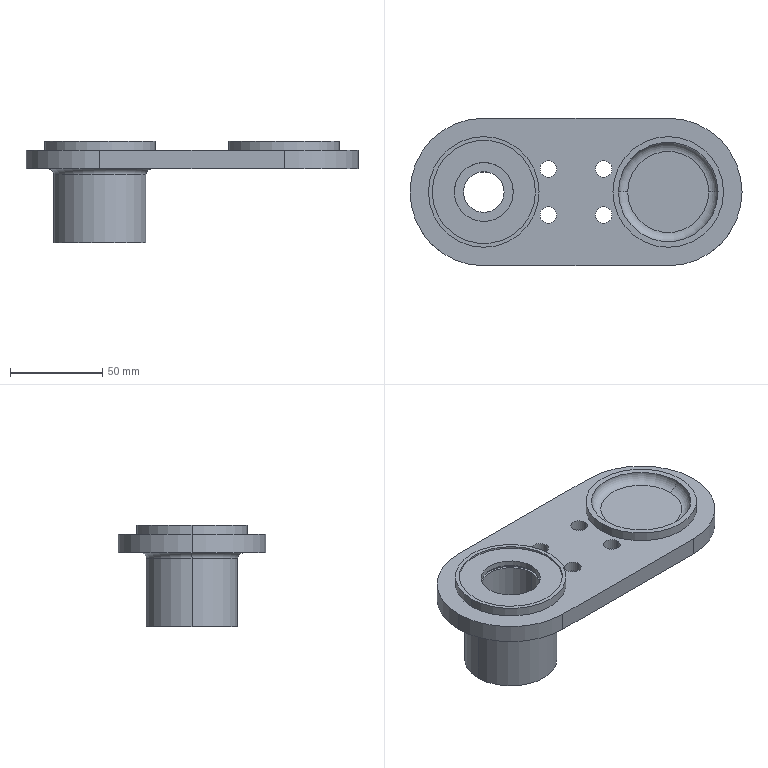Part | STEP file | Gear box plate QY-1-22 | 1 solid | 51 faces | box 180 x 80 x 55 mm | volume 179354 mm3 | cylinder 27 | plane 12 | cone 8 | torus 4 | commonest cylinder face diameters 9 x8 32 x4 60 x4 80 x3 22 x2 34.4 x2